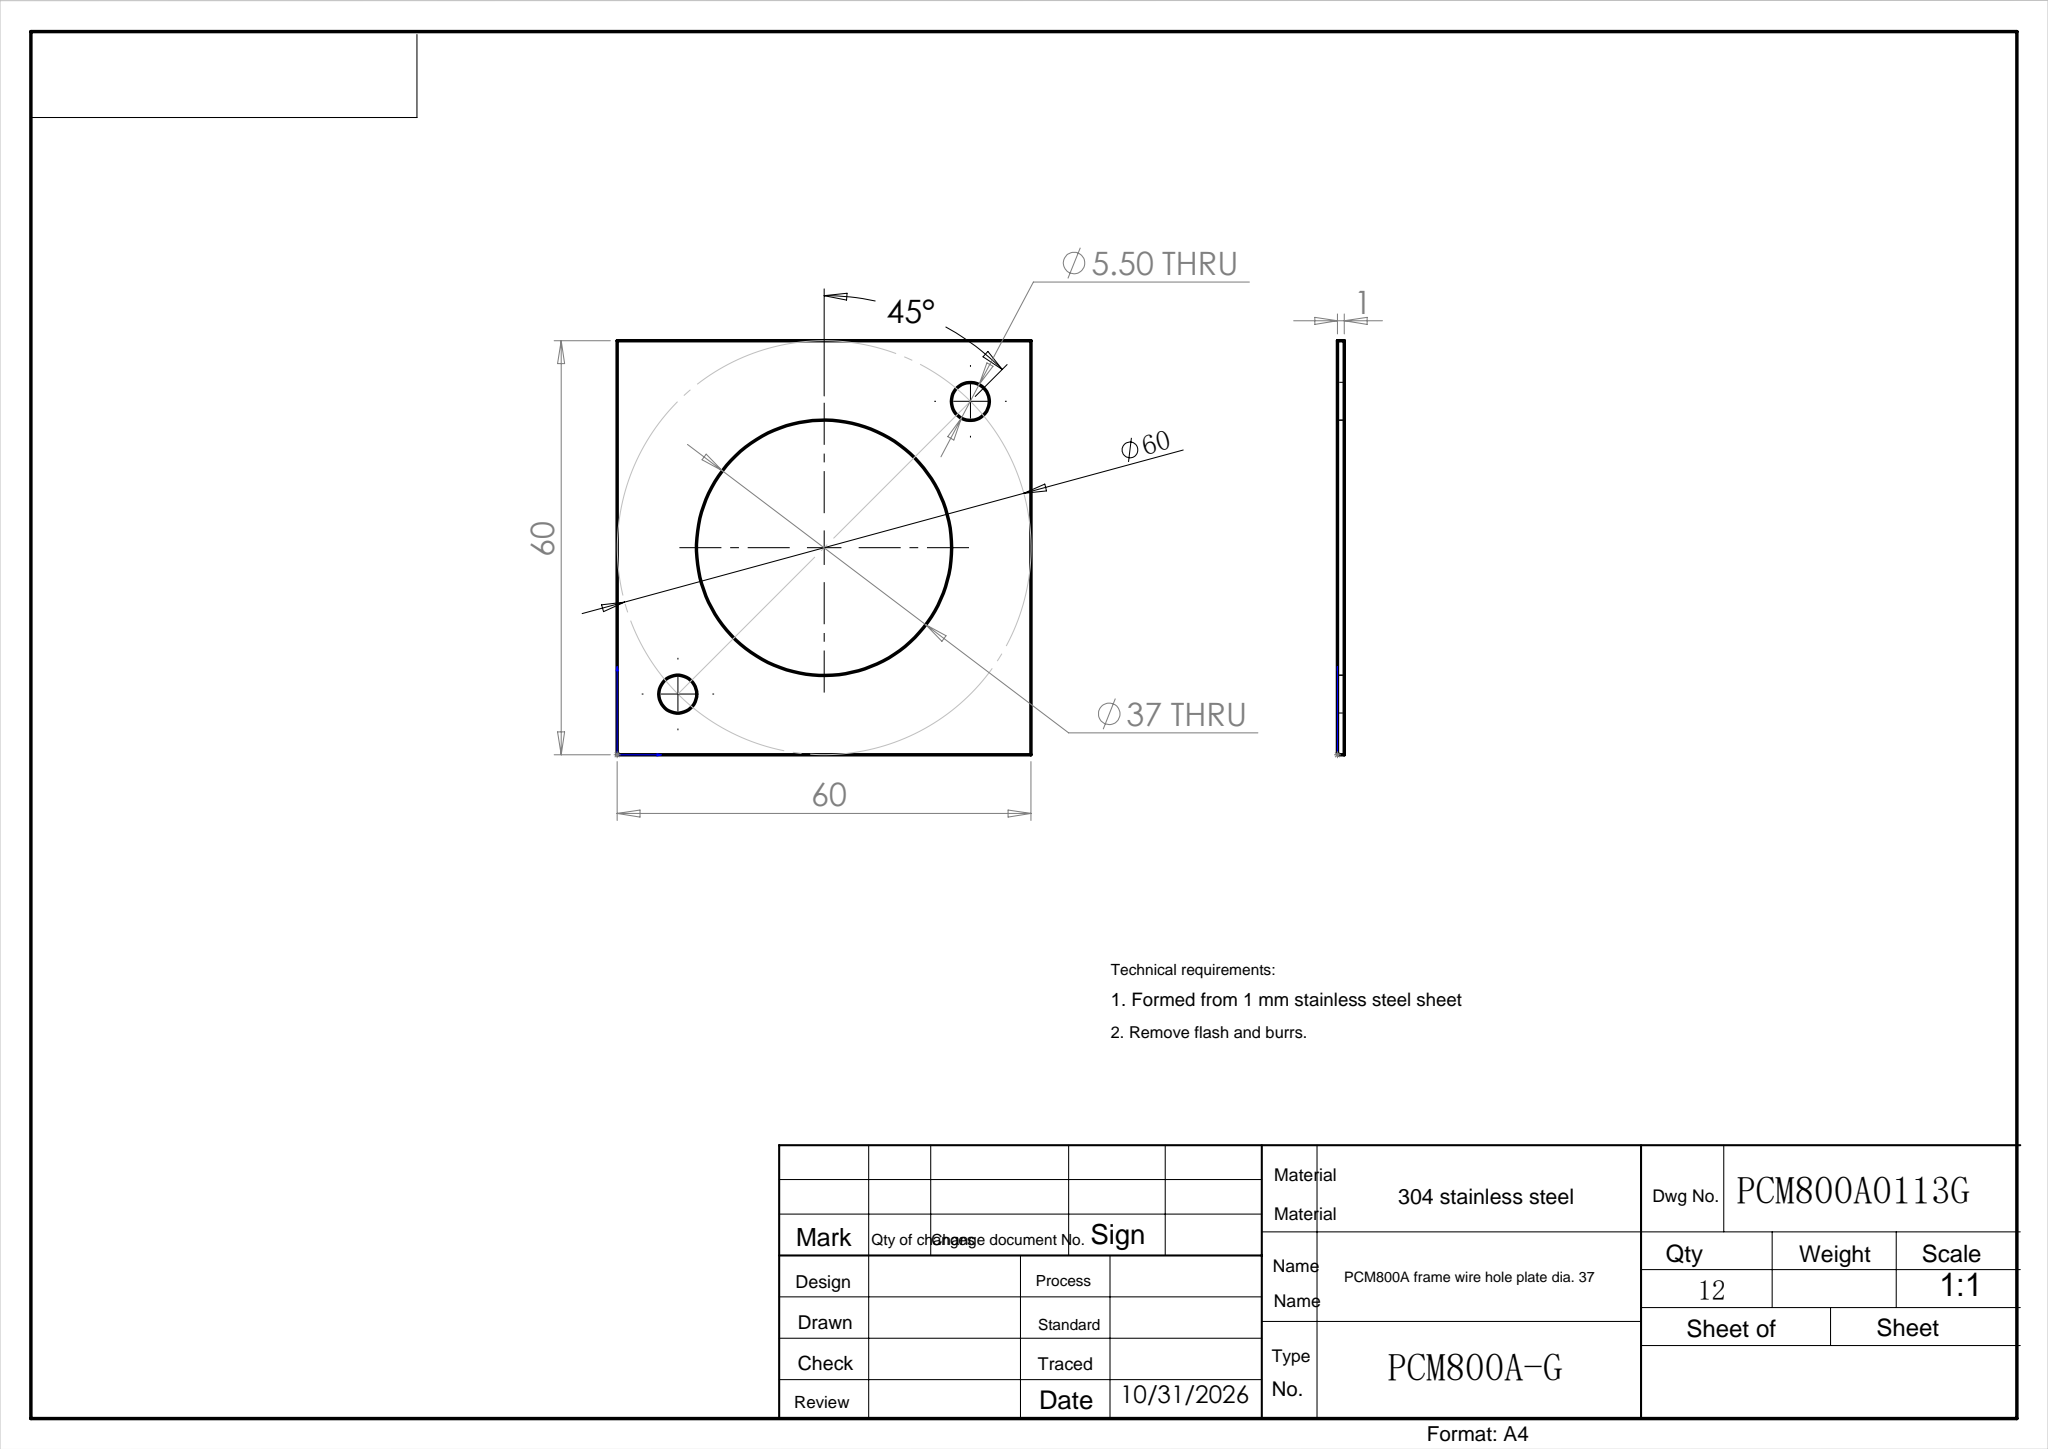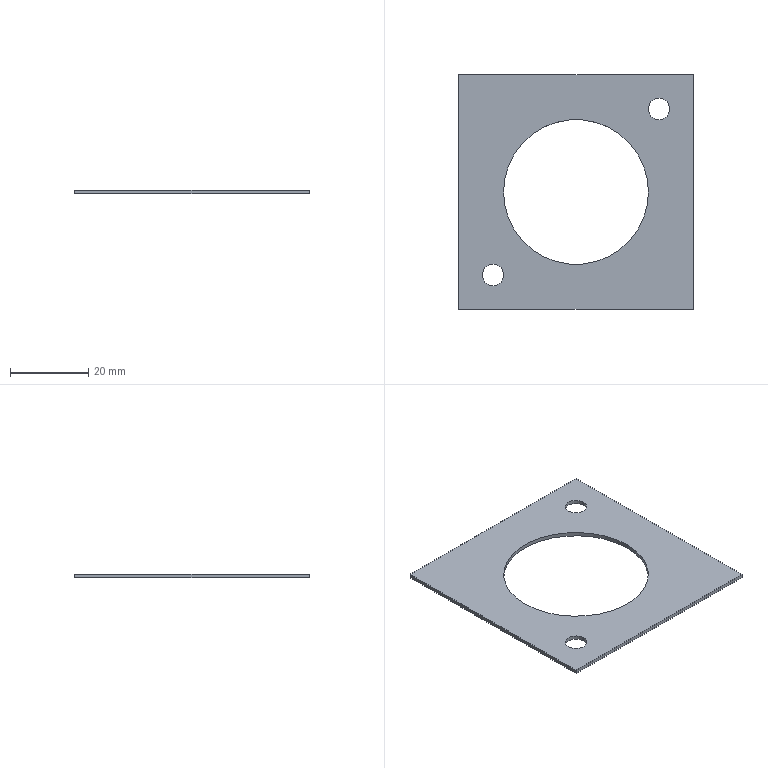Part | SolidWorks | features Extrusion 1 | 1 solid | 12 faces | box 60 x 60 x 1 mm | volume 2477 mm3 | cylinder 6 | plane 6 | commonest cylinder face diameters 5.5 x4 37 x2
STEP:
#1=CARTESIAN_POINT('',(48.463,51.213,1.));
#2=VERTEX_POINT('',#1);
#3=CARTESIAN_POINT('',(53.963,51.213,1.));
#4=VERTEX_POINT('',#3);
#5=CARTESIAN_POINT('',(51.213,51.213,1.));
#6=DIRECTION('',(0.,0.,1.));
#7=DIRECTION('',(1.,0.,0.));
#8=AXIS2_PLACEMENT_3D('',#5,#6,#7);
#9=CIRCLE('',#8,2.75);
#10=EDGE_CURVE('',#2,#4,#9,.T.);
#11=ORIENTED_EDGE('',*,*,#10,.T.);
#12=CARTESIAN_POINT('',(53.963,51.213,0.));
#13=VERTEX_POINT('',#12);
#14=CARTESIAN_POINT('',(53.963,51.213,1.));
#15=DIRECTION('',(0.,0.,-1.));
#16=VECTOR('',#15,1000.);
#17=LINE('',#14,#16);
#18=EDGE_CURVE('',#4,#13,#17,.T.);
#19=ORIENTED_EDGE('',*,*,#18,.T.);
#20=CARTESIAN_POINT('',(48.463,51.213,0.));
#21=VERTEX_POINT('',#20);
#22=CARTESIAN_POINT('',(51.213,51.213,0.));
#23=DIRECTION('',(0.,0.,1.));
#24=DIRECTION('',(1.,0.,0.));
#25=AXIS2_PLACEMENT_3D('',#22,#23,#24);
#26=CIRCLE('',#25,2.75);
#27=EDGE_CURVE('',#21,#13,#26,.T.);
#28=ORIENTED_EDGE('',*,*,#27,.F.);
#29=CARTESIAN_POINT('',(48.463,51.213,1.));
#30=DIRECTION('',(0.,0.,-1.));
#31=VECTOR('',#30,1000.);
#32=LINE('',#29,#31);
#33=EDGE_CURVE('',#2,#21,#32,.T.);
#34=ORIENTED_EDGE('',*,*,#33,.F.);
#35=EDGE_LOOP('',(#11,#19,#28,#34));
#36=FACE_OUTER_BOUND('',#35,.T.);
#37=CARTESIAN_POINT('',(51.213,51.213,1.));
#38=DIRECTION('',(0.,0.,-1.));
#39=DIRECTION('',(-1.,0.,0.));
#40=AXIS2_PLACEMENT_3D('',#37,#38,#39);
#41=CYLINDRICAL_SURFACE('',#40,2.75);
#42=ADVANCED_FACE('',(#36),#41,.F.);
#43=CARTESIAN_POINT('',(6.037,8.787,1.));
#44=VERTEX_POINT('',#43);
#45=CARTESIAN_POINT('',(11.537,8.787,1.));
#46=VERTEX_POINT('',#45);
#47=CARTESIAN_POINT('',(8.787,8.787,1.));
#48=DIRECTION('',(0.,0.,1.));
#49=DIRECTION('',(1.,0.,0.));
#50=AXIS2_PLACEMENT_3D('',#47,#48,#49);
#51=CIRCLE('',#50,2.75);
#52=EDGE_CURVE('',#44,#46,#51,.T.);
#53=ORIENTED_EDGE('',*,*,#52,.T.);
#54=CARTESIAN_POINT('',(11.537,8.787,0.));
#55=VERTEX_POINT('',#54);
#56=CARTESIAN_POINT('',(11.537,8.787,1.));
#57=DIRECTION('',(0.,0.,-1.));
#58=VECTOR('',#57,1000.);
#59=LINE('',#56,#58);
#60=EDGE_CURVE('',#46,#55,#59,.T.);
#61=ORIENTED_EDGE('',*,*,#60,.T.);
#62=CARTESIAN_POINT('',(6.037,8.787,0.));
#63=VERTEX_POINT('',#62);
#64=CARTESIAN_POINT('',(8.787,8.787,0.));
#65=DIRECTION('',(0.,0.,1.));
#66=DIRECTION('',(1.,0.,0.));
#67=AXIS2_PLACEMENT_3D('',#64,#65,#66);
#68=CIRCLE('',#67,2.75);
#69=EDGE_CURVE('',#63,#55,#68,.T.);
#70=ORIENTED_EDGE('',*,*,#69,.F.);
#71=CARTESIAN_POINT('',(6.037,8.787,1.));
#72=DIRECTION('',(0.,0.,-1.));
#73=VECTOR('',#72,1000.);
#74=LINE('',#71,#73);
#75=EDGE_CURVE('',#44,#63,#74,.T.);
#76=ORIENTED_EDGE('',*,*,#75,.F.);
#77=EDGE_LOOP('',(#53,#61,#70,#76));
#78=FACE_OUTER_BOUND('',#77,.T.);
#79=CARTESIAN_POINT('',(8.787,8.787,1.));
#80=DIRECTION('',(0.,0.,-1.));
#81=DIRECTION('',(-1.,0.,0.));
#82=AXIS2_PLACEMENT_3D('',#79,#80,#81);
#83=CYLINDRICAL_SURFACE('',#82,2.75);
#84=ADVANCED_FACE('',(#78),#83,.F.);
#85=CARTESIAN_POINT('',(11.5,30.,1.));
#86=VERTEX_POINT('',#85);
#87=CARTESIAN_POINT('',(48.5,30.,1.));
#88=VERTEX_POINT('',#87);
#89=CARTESIAN_POINT('',(30.,30.,1.));
#90=DIRECTION('',(0.,0.,1.));
#91=DIRECTION('',(1.,0.,0.));
#92=AXIS2_PLACEMENT_3D('',#89,#90,#91);
#93=CIRCLE('',#92,18.5);
#94=EDGE_CURVE('',#86,#88,#93,.T.);
#95=ORIENTED_EDGE('',*,*,#94,.T.);
#96=CARTESIAN_POINT('',(48.5,30.,0.));
#97=VERTEX_POINT('',#96);
#98=CARTESIAN_POINT('',(48.5,30.,1.));
#99=DIRECTION('',(0.,0.,-1.));
#100=VECTOR('',#99,1000.);
#101=LINE('',#98,#100);
#102=EDGE_CURVE('',#88,#97,#101,.T.);
#103=ORIENTED_EDGE('',*,*,#102,.T.);
#104=CARTESIAN_POINT('',(11.5,30.,0.));
#105=VERTEX_POINT('',#104);
#106=CARTESIAN_POINT('',(30.,30.,0.));
#107=DIRECTION('',(0.,0.,1.));
#108=DIRECTION('',(1.,0.,0.));
#109=AXIS2_PLACEMENT_3D('',#106,#107,#108);
#110=CIRCLE('',#109,18.5);
#111=EDGE_CURVE('',#105,#97,#110,.T.);
#112=ORIENTED_EDGE('',*,*,#111,.F.);
#113=CARTESIAN_POINT('',(11.5,30.,1.));
#114=DIRECTION('',(0.,0.,-1.));
#115=VECTOR('',#114,1000.);
#116=LINE('',#113,#115);
#117=EDGE_CURVE('',#86,#105,#116,.T.);
#118=ORIENTED_EDGE('',*,*,#117,.F.);
#119=EDGE_LOOP('',(#95,#103,#112,#118));
#120=FACE_OUTER_BOUND('',#119,.T.);
#121=CARTESIAN_POINT('',(30.,30.,1.));
#122=DIRECTION('',(0.,0.,-1.));
#123=DIRECTION('',(-1.,0.,0.));
#124=AXIS2_PLACEMENT_3D('',#121,#122,#123);
#125=CYLINDRICAL_SURFACE('',#124,18.5);
#126=ADVANCED_FACE('',(#120),#125,.F.);
#127=ORIENTED_EDGE('',*,*,#52,.F.);
#128=CARTESIAN_POINT('',(8.787,8.787,1.));
#129=DIRECTION('',(0.,0.,1.));
#130=DIRECTION('',(1.,0.,0.));
#131=AXIS2_PLACEMENT_3D('',#128,#129,#130);
#132=CIRCLE('',#131,2.75);
#133=EDGE_CURVE('',#46,#44,#132,.T.);
#134=ORIENTED_EDGE('',*,*,#133,.F.);
#135=EDGE_LOOP('',(#127,#134));
#136=FACE_BOUND('',#135,.T.);
#137=CARTESIAN_POINT('',(0.,60.,1.));
#138=VERTEX_POINT('',#137);
#139=CARTESIAN_POINT('',(0.,0.,1.));
#140=VERTEX_POINT('',#139);
#141=CARTESIAN_POINT('',(0.,0.,1.));
#142=DIRECTION('',(0.,-1.,0.));
#143=VECTOR('',#142,1000.);
#144=LINE('',#141,#143);
#145=EDGE_CURVE('',#138,#140,#144,.T.);
#146=ORIENTED_EDGE('',*,*,#145,.T.);
#147=CARTESIAN_POINT('',(60.,0.,1.));
#148=VERTEX_POINT('',#147);
#149=CARTESIAN_POINT('',(0.,0.,1.));
#150=DIRECTION('',(1.,0.,0.));
#151=VECTOR('',#150,1000.);
#152=LINE('',#149,#151);
#153=EDGE_CURVE('',#140,#148,#152,.T.);
#154=ORIENTED_EDGE('',*,*,#153,.T.);
#155=CARTESIAN_POINT('',(60.,60.,1.));
#156=VERTEX_POINT('',#155);
#157=CARTESIAN_POINT('',(60.,0.,1.));
#158=DIRECTION('',(0.,1.,0.));
#159=VECTOR('',#158,1000.);
#160=LINE('',#157,#159);
#161=EDGE_CURVE('',#148,#156,#160,.T.);
#162=ORIENTED_EDGE('',*,*,#161,.T.);
#163=CARTESIAN_POINT('',(0.,60.,1.));
#164=DIRECTION('',(-1.,0.,0.));
#165=VECTOR('',#164,1000.);
#166=LINE('',#163,#165);
#167=EDGE_CURVE('',#156,#138,#166,.T.);
#168=ORIENTED_EDGE('',*,*,#167,.T.);
#169=EDGE_LOOP('',(#146,#154,#162,#168));
#170=FACE_OUTER_BOUND('',#169,.T.);
#171=ORIENTED_EDGE('',*,*,#94,.F.);
#172=CARTESIAN_POINT('',(30.,30.,1.));
#173=DIRECTION('',(0.,0.,1.));
#174=DIRECTION('',(1.,0.,0.));
#175=AXIS2_PLACEMENT_3D('',#172,#173,#174);
#176=CIRCLE('',#175,18.5);
#177=EDGE_CURVE('',#88,#86,#176,.T.);
#178=ORIENTED_EDGE('',*,*,#177,.F.);
#179=EDGE_LOOP('',(#171,#178));
#180=FACE_BOUND('',#179,.T.);
#181=ORIENTED_EDGE('',*,*,#10,.F.);
#182=CARTESIAN_POINT('',(51.213,51.213,1.));
#183=DIRECTION('',(0.,0.,1.));
#184=DIRECTION('',(1.,0.,0.));
#185=AXIS2_PLACEMENT_3D('',#182,#183,#184);
#186=CIRCLE('',#185,2.75);
#187=EDGE_CURVE('',#4,#2,#186,.T.);
#188=ORIENTED_EDGE('',*,*,#187,.F.);
#189=EDGE_LOOP('',(#181,#188));
#190=FACE_BOUND('',#189,.T.);
#191=CARTESIAN_POINT('',(0.,60.,1.));
#192=DIRECTION('',(0.,0.,-1.));
#193=DIRECTION('',(-1.,0.,0.));
#194=AXIS2_PLACEMENT_3D('',#191,#192,#193);
#195=PLANE('',#194);
#196=ADVANCED_FACE('',(#136,#170,#180,#190),#195,.F.);
#197=ORIENTED_EDGE('',*,*,#69,.T.);
#198=CARTESIAN_POINT('',(8.787,8.787,0.));
#199=DIRECTION('',(0.,0.,1.));
#200=DIRECTION('',(1.,0.,0.));
#201=AXIS2_PLACEMENT_3D('',#198,#199,#200);
#202=CIRCLE('',#201,2.75);
#203=EDGE_CURVE('',#55,#63,#202,.T.);
#204=ORIENTED_EDGE('',*,*,#203,.T.);
#205=EDGE_LOOP('',(#197,#204));
#206=FACE_BOUND('',#205,.T.);
#207=CARTESIAN_POINT('',(0.,60.,0.));
#208=VERTEX_POINT('',#207);
#209=CARTESIAN_POINT('',(0.,0.,0.));
#210=VERTEX_POINT('',#209);
#211=CARTESIAN_POINT('',(0.,0.,0.));
#212=DIRECTION('',(0.,-1.,0.));
#213=VECTOR('',#212,1000.);
#214=LINE('',#211,#213);
#215=EDGE_CURVE('',#208,#210,#214,.T.);
#216=ORIENTED_EDGE('',*,*,#215,.F.);
#217=CARTESIAN_POINT('',(60.,60.,0.));
#218=VERTEX_POINT('',#217);
#219=CARTESIAN_POINT('',(0.,60.,0.));
#220=DIRECTION('',(-1.,0.,0.));
#221=VECTOR('',#220,1000.);
#222=LINE('',#219,#221);
#223=EDGE_CURVE('',#218,#208,#222,.T.);
#224=ORIENTED_EDGE('',*,*,#223,.F.);
#225=CARTESIAN_POINT('',(60.,0.,0.));
#226=VERTEX_POINT('',#225);
#227=CARTESIAN_POINT('',(60.,0.,0.));
#228=DIRECTION('',(0.,1.,0.));
#229=VECTOR('',#228,1000.);
#230=LINE('',#227,#229);
#231=EDGE_CURVE('',#226,#218,#230,.T.);
#232=ORIENTED_EDGE('',*,*,#231,.F.);
#233=CARTESIAN_POINT('',(0.,0.,0.));
#234=DIRECTION('',(1.,0.,0.));
#235=VECTOR('',#234,1000.);
#236=LINE('',#233,#235);
#237=EDGE_CURVE('',#210,#226,#236,.T.);
#238=ORIENTED_EDGE('',*,*,#237,.F.);
#239=EDGE_LOOP('',(#216,#224,#232,#238));
#240=FACE_OUTER_BOUND('',#239,.T.);
#241=ORIENTED_EDGE('',*,*,#111,.T.);
#242=CARTESIAN_POINT('',(30.,30.,0.));
#243=DIRECTION('',(0.,0.,1.));
#244=DIRECTION('',(1.,0.,0.));
#245=AXIS2_PLACEMENT_3D('',#242,#243,#244);
#246=CIRCLE('',#245,18.5);
#247=EDGE_CURVE('',#97,#105,#246,.T.);
#248=ORIENTED_EDGE('',*,*,#247,.T.);
#249=EDGE_LOOP('',(#241,#248));
#250=FACE_BOUND('',#249,.T.);
#251=ORIENTED_EDGE('',*,*,#27,.T.);
#252=CARTESIAN_POINT('',(51.213,51.213,0.));
#253=DIRECTION('',(0.,0.,1.));
#254=DIRECTION('',(1.,0.,0.));
#255=AXIS2_PLACEMENT_3D('',#252,#253,#254);
#256=CIRCLE('',#255,2.75);
#257=EDGE_CURVE('',#13,#21,#256,.T.);
#258=ORIENTED_EDGE('',*,*,#257,.T.);
#259=EDGE_LOOP('',(#251,#258));
#260=FACE_BOUND('',#259,.T.);
#261=CARTESIAN_POINT('',(0.,60.,0.));
#262=DIRECTION('',(0.,0.,-1.));
#263=DIRECTION('',(-1.,0.,0.));
#264=AXIS2_PLACEMENT_3D('',#261,#262,#263);
#265=PLANE('',#264);
#266=ADVANCED_FACE('',(#206,#240,#250,#260),#265,.T.);
#267=ORIENTED_EDGE('',*,*,#215,.T.);
#268=CARTESIAN_POINT('',(0.,0.,1.));
#269=DIRECTION('',(0.,0.,-1.));
#270=VECTOR('',#269,1000.);
#271=LINE('',#268,#270);
#272=EDGE_CURVE('',#140,#210,#271,.T.);
#273=ORIENTED_EDGE('',*,*,#272,.F.);
#274=ORIENTED_EDGE('',*,*,#145,.F.);
#275=CARTESIAN_POINT('',(0.,60.,1.));
#276=DIRECTION('',(0.,0.,-1.));
#277=VECTOR('',#276,1000.);
#278=LINE('',#275,#277);
#279=EDGE_CURVE('',#138,#208,#278,.T.);
#280=ORIENTED_EDGE('',*,*,#279,.T.);
#281=EDGE_LOOP('',(#267,#273,#274,#280));
#282=FACE_OUTER_BOUND('',#281,.T.);
#283=CARTESIAN_POINT('',(0.,0.,1.));
#284=DIRECTION('',(1.,0.,0.));
#285=DIRECTION('',(0.,1.,0.));
#286=AXIS2_PLACEMENT_3D('',#283,#284,#285);
#287=PLANE('',#286);
#288=ADVANCED_FACE('',(#282),#287,.F.);
#289=ORIENTED_EDGE('',*,*,#237,.T.);
#290=CARTESIAN_POINT('',(60.,0.,1.));
#291=DIRECTION('',(0.,0.,-1.));
#292=VECTOR('',#291,1000.);
#293=LINE('',#290,#292);
#294=EDGE_CURVE('',#148,#226,#293,.T.);
#295=ORIENTED_EDGE('',*,*,#294,.F.);
#296=ORIENTED_EDGE('',*,*,#153,.F.);
#297=ORIENTED_EDGE('',*,*,#272,.T.);
#298=EDGE_LOOP('',(#289,#295,#296,#297));
#299=FACE_OUTER_BOUND('',#298,.T.);
#300=CARTESIAN_POINT('',(0.,0.,1.));
#301=DIRECTION('',(0.,1.,0.));
#302=DIRECTION('',(0.,0.,1.));
#303=AXIS2_PLACEMENT_3D('',#300,#301,#302);
#304=PLANE('',#303);
#305=ADVANCED_FACE('',(#299),#304,.F.);
#306=ORIENTED_EDGE('',*,*,#231,.T.);
#307=CARTESIAN_POINT('',(60.,60.,1.));
#308=DIRECTION('',(0.,0.,-1.));
#309=VECTOR('',#308,1000.);
#310=LINE('',#307,#309);
#311=EDGE_CURVE('',#156,#218,#310,.T.);
#312=ORIENTED_EDGE('',*,*,#311,.F.);
#313=ORIENTED_EDGE('',*,*,#161,.F.);
#314=ORIENTED_EDGE('',*,*,#294,.T.);
#315=EDGE_LOOP('',(#306,#312,#313,#314));
#316=FACE_OUTER_BOUND('',#315,.T.);
#317=CARTESIAN_POINT('',(60.,0.,1.));
#318=DIRECTION('',(-1.,0.,0.));
#319=DIRECTION('',(0.,-1.,0.));
#320=AXIS2_PLACEMENT_3D('',#317,#318,#319);
#321=PLANE('',#320);
#322=ADVANCED_FACE('',(#316),#321,.F.);
#323=ORIENTED_EDGE('',*,*,#223,.T.);
#324=ORIENTED_EDGE('',*,*,#279,.F.);
#325=ORIENTED_EDGE('',*,*,#167,.F.);
#326=ORIENTED_EDGE('',*,*,#311,.T.);
#327=EDGE_LOOP('',(#323,#324,#325,#326));
#328=FACE_OUTER_BOUND('',#327,.T.);
#329=CARTESIAN_POINT('',(0.,60.,1.));
#330=DIRECTION('',(0.,-1.,0.));
#331=DIRECTION('',(0.,0.,-1.));
#332=AXIS2_PLACEMENT_3D('',#329,#330,#331);
#333=PLANE('',#332);
#334=ADVANCED_FACE('',(#328),#333,.F.);
#335=ORIENTED_EDGE('',*,*,#102,.F.);
#336=ORIENTED_EDGE('',*,*,#177,.T.);
#337=ORIENTED_EDGE('',*,*,#117,.T.);
#338=ORIENTED_EDGE('',*,*,#247,.F.);
#339=EDGE_LOOP('',(#335,#336,#337,#338));
#340=FACE_OUTER_BOUND('',#339,.T.);
#341=CARTESIAN_POINT('',(30.,30.,1.));
#342=DIRECTION('',(0.,0.,-1.));
#343=DIRECTION('',(-1.,0.,0.));
#344=AXIS2_PLACEMENT_3D('',#341,#342,#343);
#345=CYLINDRICAL_SURFACE('',#344,18.5);
#346=ADVANCED_FACE('',(#340),#345,.F.);
#347=ORIENTED_EDGE('',*,*,#60,.F.);
#348=ORIENTED_EDGE('',*,*,#133,.T.);
#349=ORIENTED_EDGE('',*,*,#75,.T.);
#350=ORIENTED_EDGE('',*,*,#203,.F.);
#351=EDGE_LOOP('',(#347,#348,#349,#350));
#352=FACE_OUTER_BOUND('',#351,.T.);
#353=CARTESIAN_POINT('',(8.787,8.787,1.));
#354=DIRECTION('',(0.,0.,-1.));
#355=DIRECTION('',(-1.,0.,0.));
#356=AXIS2_PLACEMENT_3D('',#353,#354,#355);
#357=CYLINDRICAL_SURFACE('',#356,2.75);
#358=ADVANCED_FACE('',(#352),#357,.F.);
#359=ORIENTED_EDGE('',*,*,#18,.F.);
#360=ORIENTED_EDGE('',*,*,#187,.T.);
#361=ORIENTED_EDGE('',*,*,#33,.T.);
#362=ORIENTED_EDGE('',*,*,#257,.F.);
#363=EDGE_LOOP('',(#359,#360,#361,#362));
#364=FACE_OUTER_BOUND('',#363,.T.);
#365=CARTESIAN_POINT('',(51.213,51.213,1.));
#366=DIRECTION('',(0.,0.,-1.));
#367=DIRECTION('',(-1.,0.,0.));
#368=AXIS2_PLACEMENT_3D('',#365,#366,#367);
#369=CYLINDRICAL_SURFACE('',#368,2.75);
#370=ADVANCED_FACE('',(#364),#369,.F.);
#371=CLOSED_SHELL('',(#42,#84,#126,#196,#266,#288,#305,#322,#334,#346,#358,#370));
#372=MANIFOLD_SOLID_BREP('',#371);
#373=CARTESIAN_POINT('',(0.,0.,0.));
#374=DIRECTION('',(0.,0.,1.));
#375=DIRECTION('',(1.,0.,0.));
#376=AXIS2_PLACEMENT_3D('',#373,#374,#375);
#377=(LENGTH_UNIT()NAMED_UNIT(*)SI_UNIT(.MILLI.,.METRE.));
#378=UNCERTAINTY_MEASURE_WITH_UNIT(LENGTH_MEASURE(0.00001),#377,'','');
#379=(NAMED_UNIT(*)PLANE_ANGLE_UNIT()SI_UNIT($,.RADIAN.));
#380=(NAMED_UNIT(*)SI_UNIT($,.STERADIAN.)SOLID_ANGLE_UNIT());
#381=(GEOMETRIC_REPRESENTATION_CONTEXT(3)GLOBAL_UNCERTAINTY_ASSIGNED_CONTEXT((#378))GLOBAL_UNIT_ASSIGNED_CONTEXT((#377,#379,#380))REPRESENTATION_CONTEXT('',''));
#382=ADVANCED_BREP_SHAPE_REPRESENTATION('',(#372,#376),#381);